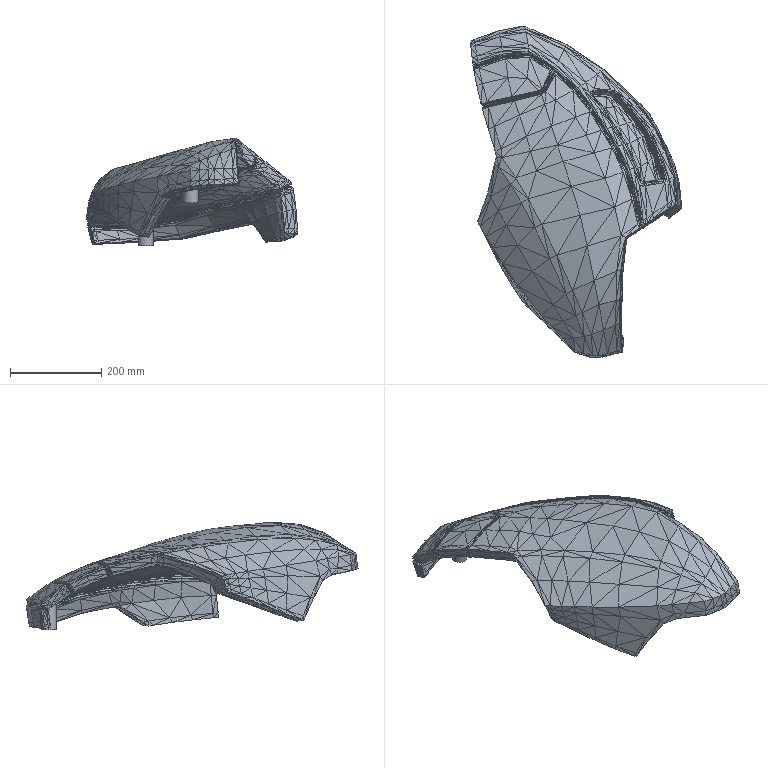Part | SolidWorks | features MirrorStock 1 | 1 solid | 2219 faces | box 464.837 x 729.145 x 237.064 mm | volume 8192368 mm3 | plane 2211 | cylinder 8 | commonest cylinder face diameters 12.5 x4 32.5 x4